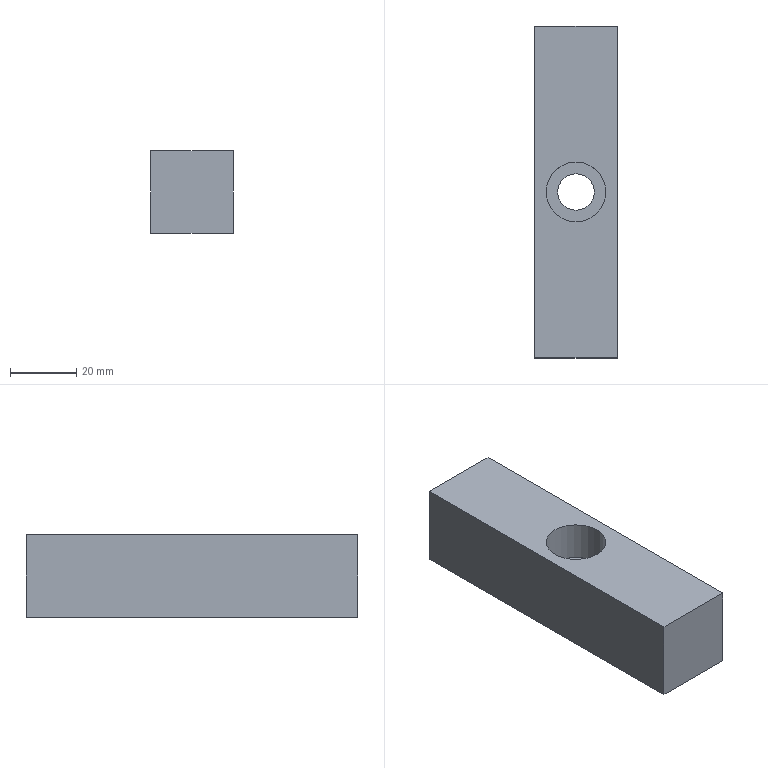Part | NX | features solid 2 | 1 solid | 9 faces | box 25 x 100 x 25 mm | volume 58211 mm3 | plane 7 | cylinder 2 | commonest cylinder face diameters 11 x1 18 x1
STEP:
#1=CARTESIAN_POINT('',(452.5,-166.513,-48.));
#2=VERTEX_POINT('',#1);
#3=CARTESIAN_POINT('',(452.5,-166.513,-73.));
#4=VERTEX_POINT('',#3);
#5=CARTESIAN_POINT('',(452.5,-166.513,-60.));
#6=DIRECTION('',(0.,0.,-1.));
#7=VECTOR('',#6,1000.);
#8=LINE('',#5,#7);
#9=EDGE_CURVE('',#2,#4,#8,.T.);
#10=ORIENTED_EDGE('',*,*,#9,.T.);
#11=CARTESIAN_POINT('',(452.5,-66.513,-73.));
#12=VERTEX_POINT('',#11);
#13=CARTESIAN_POINT('',(452.5,-166.513,-73.));
#14=DIRECTION('',(0.,1.,0.));
#15=VECTOR('',#14,1000.);
#16=LINE('',#13,#15);
#17=EDGE_CURVE('',#12,#4,#16,.F.);
#18=ORIENTED_EDGE('',*,*,#17,.F.);
#19=CARTESIAN_POINT('',(452.5,-66.513,-48.));
#20=VERTEX_POINT('',#19);
#21=CARTESIAN_POINT('',(452.5,-66.513,-60.));
#22=DIRECTION('',(0.,0.,1.));
#23=VECTOR('',#22,1000.);
#24=LINE('',#21,#23);
#25=EDGE_CURVE('',#20,#12,#24,.F.);
#26=ORIENTED_EDGE('',*,*,#25,.F.);
#27=CARTESIAN_POINT('',(452.5,-106.513,-48.));
#28=DIRECTION('',(0.,-1.,0.));
#29=VECTOR('',#28,1000.);
#30=LINE('',#27,#29);
#31=EDGE_CURVE('',#20,#2,#30,.T.);
#32=ORIENTED_EDGE('',*,*,#31,.T.);
#33=EDGE_LOOP('',(#10,#18,#26,#32));
#34=FACE_BOUND('',#33,.T.);
#35=CARTESIAN_POINT('',(452.5,-106.513,-60.));
#36=DIRECTION('',(1.,0.,0.));
#37=DIRECTION('',(0.,-1.,0.));
#38=AXIS2_PLACEMENT_3D('',#35,#36,#37);
#39=PLANE('',#38);
#40=ADVANCED_FACE('',(#34),#39,.T.);
#41=ORIENTED_EDGE('',*,*,#25,.T.);
#42=CARTESIAN_POINT('',(427.5,-66.513,-73.));
#43=VERTEX_POINT('',#42);
#44=CARTESIAN_POINT('',(452.5,-66.513,-73.));
#45=DIRECTION('',(-1.,0.,0.));
#46=VECTOR('',#45,1000.);
#47=LINE('',#44,#46);
#48=EDGE_CURVE('',#12,#43,#47,.T.);
#49=ORIENTED_EDGE('',*,*,#48,.T.);
#50=CARTESIAN_POINT('',(427.5,-66.513,-48.));
#51=VERTEX_POINT('',#50);
#52=CARTESIAN_POINT('',(427.5,-66.513,-60.));
#53=DIRECTION('',(0.,0.,-1.));
#54=VECTOR('',#53,1000.);
#55=LINE('',#52,#54);
#56=EDGE_CURVE('',#51,#43,#55,.T.);
#57=ORIENTED_EDGE('',*,*,#56,.F.);
#58=CARTESIAN_POINT('',(452.5,-66.513,-48.));
#59=DIRECTION('',(1.,0.,0.));
#60=VECTOR('',#59,1000.);
#61=LINE('',#58,#60);
#62=EDGE_CURVE('',#20,#51,#61,.F.);
#63=ORIENTED_EDGE('',*,*,#62,.F.);
#64=EDGE_LOOP('',(#41,#49,#57,#63));
#65=FACE_BOUND('',#64,.T.);
#66=CARTESIAN_POINT('',(452.5,-66.513,-60.));
#67=DIRECTION('',(0.,-1.,0.));
#68=DIRECTION('',(-1.,0.,0.));
#69=AXIS2_PLACEMENT_3D('',#66,#67,#68);
#70=PLANE('',#69);
#71=ADVANCED_FACE('',(#65),#70,.F.);
#72=ORIENTED_EDGE('',*,*,#56,.T.);
#73=CARTESIAN_POINT('',(427.5,-166.513,-73.));
#74=VERTEX_POINT('',#73);
#75=CARTESIAN_POINT('',(427.5,-106.513,-73.));
#76=DIRECTION('',(0.,-1.,0.));
#77=VECTOR('',#76,1000.);
#78=LINE('',#75,#77);
#79=EDGE_CURVE('',#43,#74,#78,.T.);
#80=ORIENTED_EDGE('',*,*,#79,.T.);
#81=CARTESIAN_POINT('',(427.5,-166.513,-48.));
#82=VERTEX_POINT('',#81);
#83=CARTESIAN_POINT('',(427.5,-166.513,-60.));
#84=DIRECTION('',(0.,0.,1.));
#85=VECTOR('',#84,1000.);
#86=LINE('',#83,#85);
#87=EDGE_CURVE('',#82,#74,#86,.F.);
#88=ORIENTED_EDGE('',*,*,#87,.F.);
#89=CARTESIAN_POINT('',(427.5,-106.513,-48.));
#90=DIRECTION('',(0.,1.,0.));
#91=VECTOR('',#90,1000.);
#92=LINE('',#89,#91);
#93=EDGE_CURVE('',#51,#82,#92,.F.);
#94=ORIENTED_EDGE('',*,*,#93,.F.);
#95=EDGE_LOOP('',(#72,#80,#88,#94));
#96=FACE_BOUND('',#95,.T.);
#97=CARTESIAN_POINT('',(427.5,-106.513,-60.));
#98=DIRECTION('',(1.,0.,0.));
#99=DIRECTION('',(0.,-1.,0.));
#100=AXIS2_PLACEMENT_3D('',#97,#98,#99);
#101=PLANE('',#100);
#102=ADVANCED_FACE('',(#96),#101,.F.);
#103=CARTESIAN_POINT('',(452.5,-166.513,-48.));
#104=DIRECTION('',(-1.,0.,0.));
#105=VECTOR('',#104,1000.);
#106=LINE('',#103,#105);
#107=EDGE_CURVE('',#2,#82,#106,.T.);
#108=ORIENTED_EDGE('',*,*,#107,.T.);
#109=ORIENTED_EDGE('',*,*,#87,.T.);
#110=CARTESIAN_POINT('',(452.5,-166.513,-73.));
#111=DIRECTION('',(1.,0.,0.));
#112=VECTOR('',#111,1000.);
#113=LINE('',#110,#112);
#114=EDGE_CURVE('',#4,#74,#113,.F.);
#115=ORIENTED_EDGE('',*,*,#114,.F.);
#116=ORIENTED_EDGE('',*,*,#9,.F.);
#117=EDGE_LOOP('',(#108,#109,#115,#116));
#118=FACE_BOUND('',#117,.T.);
#119=CARTESIAN_POINT('',(452.5,-166.513,-60.));
#120=DIRECTION('',(0.,-1.,0.));
#121=DIRECTION('',(-1.,0.,0.));
#122=AXIS2_PLACEMENT_3D('',#119,#120,#121);
#123=PLANE('',#122);
#124=ADVANCED_FACE('',(#118),#123,.T.);
#125=CARTESIAN_POINT('',(440.,-122.013,-73.));
#126=VERTEX_POINT('',#125);
#127=CARTESIAN_POINT('',(440.,-116.513,-73.));
#128=DIRECTION('',(0.,0.,1.));
#129=DIRECTION('',(0.,-1.,0.));
#130=AXIS2_PLACEMENT_3D('',#127,#128,#129);
#131=CIRCLE('',#130,5.5);
#132=EDGE_CURVE('',#126,#126,#131,.F.);
#133=ORIENTED_EDGE('',*,*,#132,.F.);
#134=EDGE_LOOP('',(#133));
#135=FACE_BOUND('',#134,.T.);
#136=ORIENTED_EDGE('',*,*,#79,.F.);
#137=ORIENTED_EDGE('',*,*,#48,.F.);
#138=ORIENTED_EDGE('',*,*,#17,.T.);
#139=ORIENTED_EDGE('',*,*,#114,.T.);
#140=EDGE_LOOP('',(#136,#137,#138,#139));
#141=FACE_BOUND('',#140,.T.);
#142=CARTESIAN_POINT('',(452.5,-166.513,-73.));
#143=DIRECTION('',(0.,0.,-1.));
#144=DIRECTION('',(-1.,0.,0.));
#145=AXIS2_PLACEMENT_3D('',#142,#143,#144);
#146=PLANE('',#145);
#147=ADVANCED_FACE('',(#135,#141),#146,.T.);
#148=CARTESIAN_POINT('',(440.,-125.513,-48.));
#149=VERTEX_POINT('',#148);
#150=CARTESIAN_POINT('',(440.,-116.513,-48.));
#151=DIRECTION('',(0.,0.,1.));
#152=DIRECTION('',(0.,-1.,0.));
#153=AXIS2_PLACEMENT_3D('',#150,#151,#152);
#154=CIRCLE('',#153,9.);
#155=EDGE_CURVE('',#149,#149,#154,.T.);
#156=ORIENTED_EDGE('',*,*,#155,.F.);
#157=EDGE_LOOP('',(#156));
#158=FACE_BOUND('',#157,.T.);
#159=ORIENTED_EDGE('',*,*,#93,.T.);
#160=ORIENTED_EDGE('',*,*,#107,.F.);
#161=ORIENTED_EDGE('',*,*,#31,.F.);
#162=ORIENTED_EDGE('',*,*,#62,.T.);
#163=EDGE_LOOP('',(#159,#160,#161,#162));
#164=FACE_BOUND('',#163,.T.);
#165=CARTESIAN_POINT('',(452.5,-106.513,-48.));
#166=DIRECTION('',(0.,0.,1.));
#167=DIRECTION('',(0.,1.,0.));
#168=AXIS2_PLACEMENT_3D('',#165,#166,#167);
#169=PLANE('',#168);
#170=ADVANCED_FACE('',(#158,#164),#169,.T.);
#171=CARTESIAN_POINT('',(440.,-122.013,-60.));
#172=VERTEX_POINT('',#171);
#173=CARTESIAN_POINT('',(440.,-116.513,-60.));
#174=DIRECTION('',(0.,0.,1.));
#175=DIRECTION('',(0.,-1.,0.));
#176=AXIS2_PLACEMENT_3D('',#173,#174,#175);
#177=CIRCLE('',#176,5.5);
#178=EDGE_CURVE('',#172,#172,#177,.T.);
#179=ORIENTED_EDGE('',*,*,#178,.T.);
#180=EDGE_LOOP('',(#179));
#181=FACE_BOUND('',#180,.T.);
#182=ORIENTED_EDGE('',*,*,#132,.T.);
#183=EDGE_LOOP('',(#182));
#184=FACE_BOUND('',#183,.T.);
#185=CARTESIAN_POINT('',(440.,-116.513,-548.));
#186=DIRECTION('',(0.,0.,-1.));
#187=DIRECTION('',(0.,-1.,0.));
#188=AXIS2_PLACEMENT_3D('',#185,#186,#187);
#189=CYLINDRICAL_SURFACE('',#188,5.5);
#190=ADVANCED_FACE('',(#181,#184),#189,.F.);
#191=ORIENTED_EDGE('',*,*,#178,.F.);
#192=EDGE_LOOP('',(#191));
#193=FACE_BOUND('',#192,.T.);
#194=CARTESIAN_POINT('',(440.,-125.513,-60.));
#195=VERTEX_POINT('',#194);
#196=CARTESIAN_POINT('',(440.,-116.513,-60.));
#197=DIRECTION('',(0.,0.,1.));
#198=DIRECTION('',(0.,-1.,0.));
#199=AXIS2_PLACEMENT_3D('',#196,#197,#198);
#200=CIRCLE('',#199,9.);
#201=EDGE_CURVE('',#195,#195,#200,.T.);
#202=ORIENTED_EDGE('',*,*,#201,.T.);
#203=EDGE_LOOP('',(#202));
#204=FACE_BOUND('',#203,.T.);
#205=CARTESIAN_POINT('',(440.,-136.513,-60.));
#206=DIRECTION('',(0.,0.,-1.));
#207=DIRECTION('',(0.,-1.,0.));
#208=AXIS2_PLACEMENT_3D('',#205,#206,#207);
#209=PLANE('',#208);
#210=ADVANCED_FACE('',(#193,#204),#209,.F.);
#211=ORIENTED_EDGE('',*,*,#201,.F.);
#212=EDGE_LOOP('',(#211));
#213=FACE_BOUND('',#212,.T.);
#214=ORIENTED_EDGE('',*,*,#155,.T.);
#215=EDGE_LOOP('',(#214));
#216=FACE_BOUND('',#215,.T.);
#217=CARTESIAN_POINT('',(440.,-116.513,-48.));
#218=DIRECTION('',(0.,0.,-1.));
#219=DIRECTION('',(0.,-1.,0.));
#220=AXIS2_PLACEMENT_3D('',#217,#218,#219);
#221=CYLINDRICAL_SURFACE('',#220,9.);
#222=ADVANCED_FACE('',(#213,#216),#221,.F.);
#223=CLOSED_SHELL('',(#40,#71,#102,#124,#147,#170,#190,#210,#222));
#224=MANIFOLD_SOLID_BREP('',#223);
#225=(LENGTH_UNIT()NAMED_UNIT(*)SI_UNIT(.MILLI.,.METRE.));
#226=UNCERTAINTY_MEASURE_WITH_UNIT(LENGTH_MEASURE(0.00001),#225,'','');
#227=(NAMED_UNIT(*)PLANE_ANGLE_UNIT()SI_UNIT($,.RADIAN.));
#228=(NAMED_UNIT(*)SI_UNIT($,.STERADIAN.)SOLID_ANGLE_UNIT());
#229=(GEOMETRIC_REPRESENTATION_CONTEXT(3)GLOBAL_UNCERTAINTY_ASSIGNED_CONTEXT((#226))GLOBAL_UNIT_ASSIGNED_CONTEXT((#225,#227,#228))REPRESENTATION_CONTEXT('',''));
#230=ADVANCED_BREP_SHAPE_REPRESENTATION('',(#224),#229);